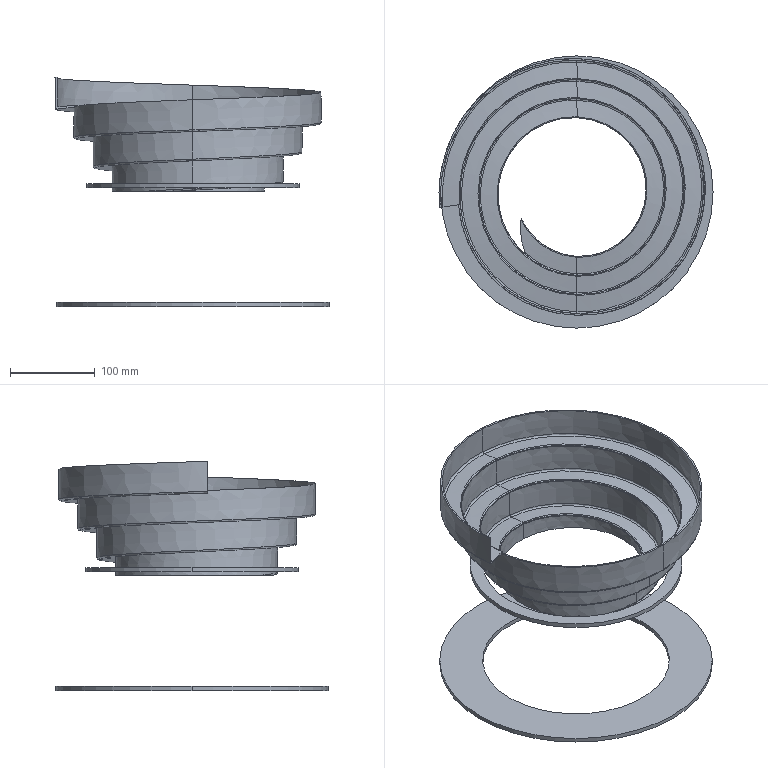Part | STEP file | 222_4 | 3 solids | 108 faces | box 322.673 x 320.624 x 270.209 mm | volume 556791 mm3 | spline 93 | cylinder 8 | plane 7 | commonest cylinder face diameters 220 x4 250 x2 320.624 x2